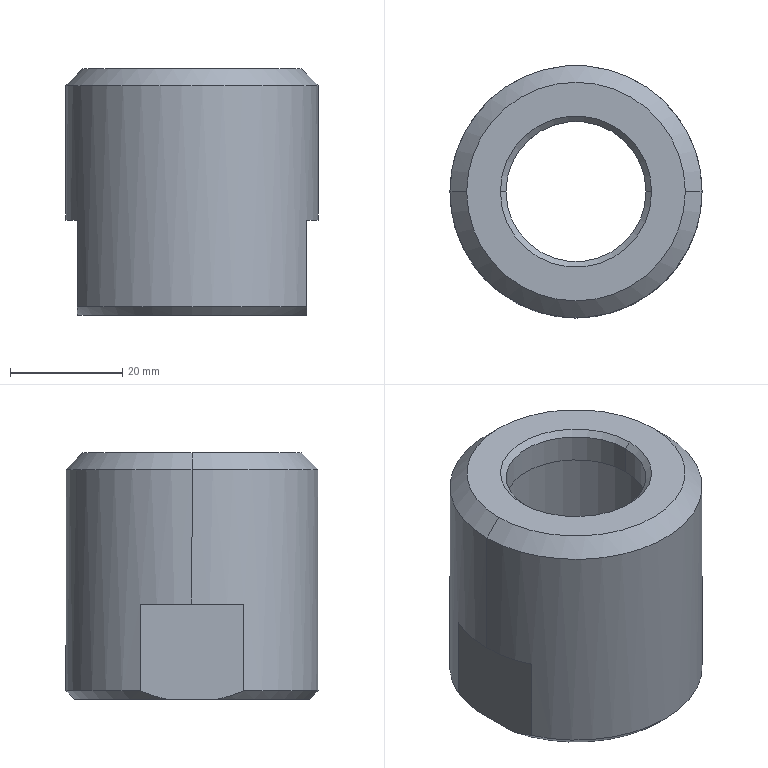Part | SolidWorks | features BaseBody 1 | 1 solid | 24 faces | box 45 x 45 x 44 mm | volume 29973 mm3 | cylinder 8 | cone 8 | plane 8 | commonest cylinder face diameters 25 x2 34.376 x2 34.5 x2 45 x2
STEP:
#1=CARTESIAN_POINT('',(-20.5,9.274,-27.));
#2=VERTEX_POINT('',#1);
#3=CARTESIAN_POINT('',(-22.5,0.,-27.));
#4=VERTEX_POINT('',#3);
#5=CARTESIAN_POINT('',(0.,0.,-27.));
#6=DIRECTION('',(0.,0.,1.));
#7=DIRECTION('',(1.,0.,0.));
#8=AXIS2_PLACEMENT_3D('',#5,#6,#7);
#9=CIRCLE('',#8,22.5);
#10=EDGE_CURVE('',#2,#4,#9,.T.);
#11=ORIENTED_EDGE('',*,*,#10,.T.);
#12=CARTESIAN_POINT('',(-22.5,0.,-3.));
#13=VERTEX_POINT('',#12);
#14=CARTESIAN_POINT('',(-22.5,0.,-44.));
#15=DIRECTION('',(0.,0.,1.));
#16=VECTOR('',#15,1000.);
#17=LINE('',#14,#16);
#18=EDGE_CURVE('',#4,#13,#17,.T.);
#19=ORIENTED_EDGE('',*,*,#18,.T.);
#20=CARTESIAN_POINT('',(22.5,0.,-3.));
#21=VERTEX_POINT('',#20);
#22=CARTESIAN_POINT('',(0.,0.,-3.));
#23=DIRECTION('',(0.,0.,-1.));
#24=DIRECTION('',(1.,0.,0.));
#25=AXIS2_PLACEMENT_3D('',#22,#23,#24);
#26=CIRCLE('',#25,22.5);
#27=EDGE_CURVE('',#13,#21,#26,.T.);
#28=ORIENTED_EDGE('',*,*,#27,.T.);
#29=CARTESIAN_POINT('',(22.5,0.,-27.));
#30=VERTEX_POINT('',#29);
#31=CARTESIAN_POINT('',(22.5,0.,-44.));
#32=DIRECTION('',(0.,0.,1.));
#33=VECTOR('',#32,1000.);
#34=LINE('',#31,#33);
#35=EDGE_CURVE('',#30,#21,#34,.T.);
#36=ORIENTED_EDGE('',*,*,#35,.F.);
#37=CARTESIAN_POINT('',(20.5,9.274,-27.));
#38=VERTEX_POINT('',#37);
#39=CARTESIAN_POINT('',(0.,0.,-27.));
#40=DIRECTION('',(0.,0.,1.));
#41=DIRECTION('',(1.,0.,0.));
#42=AXIS2_PLACEMENT_3D('',#39,#40,#41);
#43=CIRCLE('',#42,22.5);
#44=EDGE_CURVE('',#30,#38,#43,.T.);
#45=ORIENTED_EDGE('',*,*,#44,.T.);
#46=CARTESIAN_POINT('',(20.5,9.274,-42.5));
#47=VERTEX_POINT('',#46);
#48=CARTESIAN_POINT('',(20.5,9.274,-44.));
#49=DIRECTION('',(0.,0.,-1.));
#50=VECTOR('',#49,1000.);
#51=LINE('',#48,#50);
#52=EDGE_CURVE('',#38,#47,#51,.T.);
#53=ORIENTED_EDGE('',*,*,#52,.T.);
#54=CARTESIAN_POINT('',(-20.5,9.274,-42.5));
#55=VERTEX_POINT('',#54);
#56=CARTESIAN_POINT('',(0.,0.,-42.5));
#57=DIRECTION('',(0.,0.,1.));
#58=DIRECTION('',(1.,0.,0.));
#59=AXIS2_PLACEMENT_3D('',#56,#57,#58);
#60=CIRCLE('',#59,22.5);
#61=EDGE_CURVE('',#47,#55,#60,.T.);
#62=ORIENTED_EDGE('',*,*,#61,.T.);
#63=CARTESIAN_POINT('',(-20.5,9.274,-44.));
#64=DIRECTION('',(0.,0.,1.));
#65=VECTOR('',#64,1000.);
#66=LINE('',#63,#65);
#67=EDGE_CURVE('',#55,#2,#66,.T.);
#68=ORIENTED_EDGE('',*,*,#67,.T.);
#69=EDGE_LOOP('',(#11,#19,#28,#36,#45,#53,#62,#68));
#70=FACE_OUTER_BOUND('',#69,.T.);
#71=CARTESIAN_POINT('',(0.,0.,-44.));
#72=DIRECTION('',(0.,0.,1.));
#73=DIRECTION('',(1.,0.,0.));
#74=AXIS2_PLACEMENT_3D('',#71,#72,#73);
#75=CYLINDRICAL_SURFACE('',#74,22.5);
#76=ADVANCED_FACE('',(#70),#75,.T.);
#77=CARTESIAN_POINT('',(-19.5,0.,0.));
#78=VERTEX_POINT('',#77);
#79=CARTESIAN_POINT('',(19.5,0.,0.));
#80=VERTEX_POINT('',#79);
#81=CARTESIAN_POINT('',(0.,0.,0.));
#82=DIRECTION('',(0.,0.,-1.));
#83=DIRECTION('',(-1.,0.,0.));
#84=AXIS2_PLACEMENT_3D('',#81,#82,#83);
#85=CIRCLE('',#84,19.5);
#86=EDGE_CURVE('',#78,#80,#85,.T.);
#87=ORIENTED_EDGE('',*,*,#86,.T.);
#88=CARTESIAN_POINT('',(22.5,0.,-3.));
#89=DIRECTION('',(0.7071,0.,-0.7071));
#90=VECTOR('',#89,1000.);
#91=LINE('',#88,#90);
#92=EDGE_CURVE('',#80,#21,#91,.T.);
#93=ORIENTED_EDGE('',*,*,#92,.T.);
#94=ORIENTED_EDGE('',*,*,#27,.F.);
#95=CARTESIAN_POINT('',(-22.5,0.,-3.));
#96=DIRECTION('',(-0.7071,0.,-0.7071));
#97=VECTOR('',#96,1000.);
#98=LINE('',#95,#97);
#99=EDGE_CURVE('',#78,#13,#98,.T.);
#100=ORIENTED_EDGE('',*,*,#99,.F.);
#101=EDGE_LOOP('',(#87,#93,#94,#100));
#102=FACE_OUTER_BOUND('',#101,.T.);
#103=CARTESIAN_POINT('',(0.,0.,-3.));
#104=DIRECTION('',(0.,0.,-1.));
#105=DIRECTION('',(-1.,0.,0.));
#106=AXIS2_PLACEMENT_3D('',#103,#104,#105);
#107=CONICAL_SURFACE('',#106,22.5,0.7854);
#108=ADVANCED_FACE('',(#102),#107,.T.);
#109=CARTESIAN_POINT('',(17.188,0.,-43.188));
#110=VERTEX_POINT('',#109);
#111=CARTESIAN_POINT('',(-17.188,0.,-43.188));
#112=VERTEX_POINT('',#111);
#113=CARTESIAN_POINT('',(0.,0.,-43.188));
#114=DIRECTION('',(0.,0.,-1.));
#115=DIRECTION('',(-1.,0.,0.));
#116=AXIS2_PLACEMENT_3D('',#113,#114,#115);
#117=CIRCLE('',#116,17.188);
#118=EDGE_CURVE('',#110,#112,#117,.T.);
#119=ORIENTED_EDGE('',*,*,#118,.F.);
#120=CARTESIAN_POINT('',(18.,0.,-44.));
#121=VERTEX_POINT('',#120);
#122=CARTESIAN_POINT('',(18.,0.,-44.));
#123=DIRECTION('',(0.7071,0.,-0.7071));
#124=VECTOR('',#123,1000.);
#125=LINE('',#122,#124);
#126=EDGE_CURVE('',#110,#121,#125,.T.);
#127=ORIENTED_EDGE('',*,*,#126,.T.);
#128=CARTESIAN_POINT('',(-18.,0.,-44.));
#129=VERTEX_POINT('',#128);
#130=CARTESIAN_POINT('',(0.,0.,-44.));
#131=DIRECTION('',(0.,0.,1.));
#132=DIRECTION('',(-1.,0.,0.));
#133=AXIS2_PLACEMENT_3D('',#130,#131,#132);
#134=CIRCLE('',#133,18.);
#135=EDGE_CURVE('',#129,#121,#134,.T.);
#136=ORIENTED_EDGE('',*,*,#135,.F.);
#137=CARTESIAN_POINT('',(-18.,0.,-44.));
#138=DIRECTION('',(-0.7071,0.,-0.7071));
#139=VECTOR('',#138,1000.);
#140=LINE('',#137,#139);
#141=EDGE_CURVE('',#112,#129,#140,.T.);
#142=ORIENTED_EDGE('',*,*,#141,.F.);
#143=EDGE_LOOP('',(#119,#127,#136,#142));
#144=FACE_OUTER_BOUND('',#143,.T.);
#145=CARTESIAN_POINT('',(0.,0.,-44.));
#146=DIRECTION('',(0.,0.,-1.));
#147=DIRECTION('',(-1.,0.,0.));
#148=AXIS2_PLACEMENT_3D('',#145,#146,#147);
#149=CONICAL_SURFACE('',#148,18.,0.7854);
#150=ADVANCED_FACE('',(#144),#149,.F.);
#151=CARTESIAN_POINT('',(-12.5,0.,-1.));
#152=VERTEX_POINT('',#151);
#153=CARTESIAN_POINT('',(12.5,0.,-1.));
#154=VERTEX_POINT('',#153);
#155=CARTESIAN_POINT('',(0.,0.,-1.));
#156=DIRECTION('',(0.,0.,1.));
#157=DIRECTION('',(1.,0.,0.));
#158=AXIS2_PLACEMENT_3D('',#155,#156,#157);
#159=CIRCLE('',#158,12.5);
#160=EDGE_CURVE('',#152,#154,#159,.T.);
#161=ORIENTED_EDGE('',*,*,#160,.F.);
#162=CARTESIAN_POINT('',(-13.5,0.,0.));
#163=VERTEX_POINT('',#162);
#164=CARTESIAN_POINT('',(-13.5,0.,0.));
#165=DIRECTION('',(-0.7071,0.,0.7071));
#166=VECTOR('',#165,1000.);
#167=LINE('',#164,#166);
#168=EDGE_CURVE('',#152,#163,#167,.T.);
#169=ORIENTED_EDGE('',*,*,#168,.T.);
#170=CARTESIAN_POINT('',(13.5,0.,0.));
#171=VERTEX_POINT('',#170);
#172=CARTESIAN_POINT('',(0.,0.,0.));
#173=DIRECTION('',(0.,0.,-1.));
#174=DIRECTION('',(1.,0.,0.));
#175=AXIS2_PLACEMENT_3D('',#172,#173,#174);
#176=CIRCLE('',#175,13.5);
#177=EDGE_CURVE('',#171,#163,#176,.T.);
#178=ORIENTED_EDGE('',*,*,#177,.F.);
#179=CARTESIAN_POINT('',(13.5,0.,0.));
#180=DIRECTION('',(0.7071,0.,0.7071));
#181=VECTOR('',#180,1000.);
#182=LINE('',#179,#181);
#183=EDGE_CURVE('',#154,#171,#182,.T.);
#184=ORIENTED_EDGE('',*,*,#183,.F.);
#185=EDGE_LOOP('',(#161,#169,#178,#184));
#186=FACE_OUTER_BOUND('',#185,.T.);
#187=CARTESIAN_POINT('',(0.,0.,0.));
#188=DIRECTION('',(0.,0.,1.));
#189=DIRECTION('',(1.,0.,0.));
#190=AXIS2_PLACEMENT_3D('',#187,#188,#189);
#191=CONICAL_SURFACE('',#190,13.5,0.7854);
#192=ADVANCED_FACE('',(#186),#191,.F.);
#193=ORIENTED_EDGE('',*,*,#118,.T.);
#194=CARTESIAN_POINT('',(-17.188,0.,-27.));
#195=VERTEX_POINT('',#194);
#196=CARTESIAN_POINT('',(-17.188,0.,-44.));
#197=DIRECTION('',(0.,0.,1.));
#198=VECTOR('',#197,1000.);
#199=LINE('',#196,#198);
#200=EDGE_CURVE('',#112,#195,#199,.T.);
#201=ORIENTED_EDGE('',*,*,#200,.T.);
#202=CARTESIAN_POINT('',(17.188,0.,-27.));
#203=VERTEX_POINT('',#202);
#204=CARTESIAN_POINT('',(0.,0.,-27.));
#205=DIRECTION('',(0.,0.,-1.));
#206=DIRECTION('',(1.,0.,0.));
#207=AXIS2_PLACEMENT_3D('',#204,#205,#206);
#208=CIRCLE('',#207,17.188);
#209=EDGE_CURVE('',#203,#195,#208,.T.);
#210=ORIENTED_EDGE('',*,*,#209,.F.);
#211=CARTESIAN_POINT('',(17.188,0.,-44.));
#212=DIRECTION('',(0.,0.,1.));
#213=VECTOR('',#212,1000.);
#214=LINE('',#211,#213);
#215=EDGE_CURVE('',#110,#203,#214,.T.);
#216=ORIENTED_EDGE('',*,*,#215,.F.);
#217=EDGE_LOOP('',(#193,#201,#210,#216));
#218=FACE_OUTER_BOUND('',#217,.T.);
#219=CARTESIAN_POINT('',(0.,0.,-44.));
#220=DIRECTION('',(0.,0.,1.));
#221=DIRECTION('',(1.,0.,0.));
#222=AXIS2_PLACEMENT_3D('',#219,#220,#221);
#223=CYLINDRICAL_SURFACE('',#222,17.188);
#224=ADVANCED_FACE('',(#218),#223,.F.);
#225=CARTESIAN_POINT('',(-12.5,0.,-6.));
#226=VERTEX_POINT('',#225);
#227=CARTESIAN_POINT('',(12.5,0.,-6.));
#228=VERTEX_POINT('',#227);
#229=CARTESIAN_POINT('',(0.,0.,-6.));
#230=DIRECTION('',(0.,0.,1.));
#231=DIRECTION('',(1.,0.,0.));
#232=AXIS2_PLACEMENT_3D('',#229,#230,#231);
#233=CIRCLE('',#232,12.5);
#234=EDGE_CURVE('',#226,#228,#233,.T.);
#235=ORIENTED_EDGE('',*,*,#234,.F.);
#236=CARTESIAN_POINT('',(-12.5,0.,-44.));
#237=DIRECTION('',(0.,0.,1.));
#238=VECTOR('',#237,1000.);
#239=LINE('',#236,#238);
#240=EDGE_CURVE('',#226,#152,#239,.T.);
#241=ORIENTED_EDGE('',*,*,#240,.T.);
#242=ORIENTED_EDGE('',*,*,#160,.T.);
#243=CARTESIAN_POINT('',(12.5,0.,-44.));
#244=DIRECTION('',(0.,0.,1.));
#245=VECTOR('',#244,1000.);
#246=LINE('',#243,#245);
#247=EDGE_CURVE('',#228,#154,#246,.T.);
#248=ORIENTED_EDGE('',*,*,#247,.F.);
#249=EDGE_LOOP('',(#235,#241,#242,#248));
#250=FACE_OUTER_BOUND('',#249,.T.);
#251=CARTESIAN_POINT('',(0.,0.,-44.));
#252=DIRECTION('',(0.,0.,1.));
#253=DIRECTION('',(1.,0.,0.));
#254=AXIS2_PLACEMENT_3D('',#251,#252,#253);
#255=CYLINDRICAL_SURFACE('',#254,12.5);
#256=ADVANCED_FACE('',(#250),#255,.F.);
#257=CARTESIAN_POINT('',(-17.25,0.,-27.));
#258=VERTEX_POINT('',#257);
#259=CARTESIAN_POINT('',(17.25,0.,-27.));
#260=VERTEX_POINT('',#259);
#261=CARTESIAN_POINT('',(0.,0.,-27.));
#262=DIRECTION('',(0.,0.,1.));
#263=DIRECTION('',(1.,0.,0.));
#264=AXIS2_PLACEMENT_3D('',#261,#262,#263);
#265=CIRCLE('',#264,17.25);
#266=EDGE_CURVE('',#258,#260,#265,.T.);
#267=ORIENTED_EDGE('',*,*,#266,.F.);
#268=CARTESIAN_POINT('',(-17.25,0.,-6.));
#269=VERTEX_POINT('',#268);
#270=CARTESIAN_POINT('',(-17.25,0.,-44.));
#271=DIRECTION('',(0.,0.,1.));
#272=VECTOR('',#271,1000.);
#273=LINE('',#270,#272);
#274=EDGE_CURVE('',#258,#269,#273,.T.);
#275=ORIENTED_EDGE('',*,*,#274,.T.);
#276=CARTESIAN_POINT('',(17.25,0.,-6.));
#277=VERTEX_POINT('',#276);
#278=CARTESIAN_POINT('',(0.,0.,-6.));
#279=DIRECTION('',(0.,0.,-1.));
#280=DIRECTION('',(1.,0.,0.));
#281=AXIS2_PLACEMENT_3D('',#278,#279,#280);
#282=CIRCLE('',#281,17.25);
#283=EDGE_CURVE('',#277,#269,#282,.T.);
#284=ORIENTED_EDGE('',*,*,#283,.F.);
#285=CARTESIAN_POINT('',(17.25,0.,-44.));
#286=DIRECTION('',(0.,0.,1.));
#287=VECTOR('',#286,1000.);
#288=LINE('',#285,#287);
#289=EDGE_CURVE('',#260,#277,#288,.T.);
#290=ORIENTED_EDGE('',*,*,#289,.F.);
#291=EDGE_LOOP('',(#267,#275,#284,#290));
#292=FACE_OUTER_BOUND('',#291,.T.);
#293=CARTESIAN_POINT('',(0.,0.,-44.));
#294=DIRECTION('',(0.,0.,1.));
#295=DIRECTION('',(1.,0.,0.));
#296=AXIS2_PLACEMENT_3D('',#293,#294,#295);
#297=CYLINDRICAL_SURFACE('',#296,17.25);
#298=ADVANCED_FACE('',(#292),#297,.F.);
#299=ORIENTED_EDGE('',*,*,#18,.F.);
#300=CARTESIAN_POINT('',(-20.5,-9.274,-27.));
#301=VERTEX_POINT('',#300);
#302=CARTESIAN_POINT('',(0.,0.,-27.));
#303=DIRECTION('',(0.,0.,1.));
#304=DIRECTION('',(1.,0.,0.));
#305=AXIS2_PLACEMENT_3D('',#302,#303,#304);
#306=CIRCLE('',#305,22.5);
#307=EDGE_CURVE('',#4,#301,#306,.T.);
#308=ORIENTED_EDGE('',*,*,#307,.T.);
#309=CARTESIAN_POINT('',(-20.5,-9.274,-42.5));
#310=VERTEX_POINT('',#309);
#311=CARTESIAN_POINT('',(-20.5,-9.274,-44.));
#312=DIRECTION('',(0.,0.,-1.));
#313=VECTOR('',#312,1000.);
#314=LINE('',#311,#313);
#315=EDGE_CURVE('',#301,#310,#314,.T.);
#316=ORIENTED_EDGE('',*,*,#315,.T.);
#317=CARTESIAN_POINT('',(20.5,-9.274,-42.5));
#318=VERTEX_POINT('',#317);
#319=CARTESIAN_POINT('',(0.,0.,-42.5));
#320=DIRECTION('',(0.,0.,1.));
#321=DIRECTION('',(1.,0.,0.));
#322=AXIS2_PLACEMENT_3D('',#319,#320,#321);
#323=CIRCLE('',#322,22.5);
#324=EDGE_CURVE('',#310,#318,#323,.T.);
#325=ORIENTED_EDGE('',*,*,#324,.T.);
#326=CARTESIAN_POINT('',(20.5,-9.274,-27.));
#327=VERTEX_POINT('',#326);
#328=CARTESIAN_POINT('',(20.5,-9.274,-44.));
#329=DIRECTION('',(0.,0.,1.));
#330=VECTOR('',#329,1000.);
#331=LINE('',#328,#330);
#332=EDGE_CURVE('',#318,#327,#331,.T.);
#333=ORIENTED_EDGE('',*,*,#332,.T.);
#334=CARTESIAN_POINT('',(0.,0.,-27.));
#335=DIRECTION('',(0.,0.,1.));
#336=DIRECTION('',(1.,0.,0.));
#337=AXIS2_PLACEMENT_3D('',#334,#335,#336);
#338=CIRCLE('',#337,22.5);
#339=EDGE_CURVE('',#327,#30,#338,.T.);
#340=ORIENTED_EDGE('',*,*,#339,.T.);
#341=ORIENTED_EDGE('',*,*,#35,.T.);
#342=CARTESIAN_POINT('',(0.,0.,-3.));
#343=DIRECTION('',(0.,0.,-1.));
#344=DIRECTION('',(1.,0.,0.));
#345=AXIS2_PLACEMENT_3D('',#342,#343,#344);
#346=CIRCLE('',#345,22.5);
#347=EDGE_CURVE('',#21,#13,#346,.T.);
#348=ORIENTED_EDGE('',*,*,#347,.T.);
#349=EDGE_LOOP('',(#299,#308,#316,#325,#333,#340,#341,#348));
#350=FACE_OUTER_BOUND('',#349,.T.);
#351=CARTESIAN_POINT('',(0.,0.,-44.));
#352=DIRECTION('',(0.,0.,1.));
#353=DIRECTION('',(1.,0.,0.));
#354=AXIS2_PLACEMENT_3D('',#351,#352,#353);
#355=CYLINDRICAL_SURFACE('',#354,22.5);
#356=ADVANCED_FACE('',(#350),#355,.T.);
#357=CARTESIAN_POINT('',(20.5,30.,-27.));
#358=DIRECTION('',(0.,-1.,0.));
#359=VECTOR('',#358,1000.);
#360=LINE('',#357,#359);
#361=EDGE_CURVE('',#38,#327,#360,.T.);
#362=ORIENTED_EDGE('',*,*,#361,.T.);
#363=ORIENTED_EDGE('',*,*,#332,.F.);
#364=CARTESIAN_POINT('',(20.5,-4.555,-44.));
#365=VERTEX_POINT('',#364);
#366=CARTESIAN_POINT('',(20.5,-9.274,-42.5));
#367=CARTESIAN_POINT('',(20.5,-7.742,-43.131));
#368=CARTESIAN_POINT('',(20.5,-6.175,-43.649));
#369=CARTESIAN_POINT('',(20.5,-4.555,-44.));
#370=B_SPLINE_CURVE_WITH_KNOTS('',3,(#366,#367,#368,#369),.UNSPECIFIED.,.F.,.F.,(4,4),(0.,0.004951),.UNSPECIFIED.);
#371=EDGE_CURVE('',#318,#365,#370,.T.);
#372=ORIENTED_EDGE('',*,*,#371,.T.);
#373=CARTESIAN_POINT('',(20.5,4.555,-44.));
#374=VERTEX_POINT('',#373);
#375=CARTESIAN_POINT('',(20.5,30.,-44.));
#376=DIRECTION('',(0.,1.,0.));
#377=VECTOR('',#376,1000.);
#378=LINE('',#375,#377);
#379=EDGE_CURVE('',#365,#374,#378,.T.);
#380=ORIENTED_EDGE('',*,*,#379,.T.);
#381=CARTESIAN_POINT('',(20.5,4.555,-44.));
#382=CARTESIAN_POINT('',(20.5,6.175,-43.649));
#383=CARTESIAN_POINT('',(20.5,7.742,-43.131));
#384=CARTESIAN_POINT('',(20.5,9.274,-42.5));
#385=B_SPLINE_CURVE_WITH_KNOTS('',3,(#381,#382,#383,#384),.UNSPECIFIED.,.F.,.F.,(4,4),(0.,0.004951),.UNSPECIFIED.);
#386=EDGE_CURVE('',#374,#47,#385,.T.);
#387=ORIENTED_EDGE('',*,*,#386,.T.);
#388=ORIENTED_EDGE('',*,*,#52,.F.);
#389=EDGE_LOOP('',(#362,#363,#372,#380,#387,#388));
#390=FACE_OUTER_BOUND('',#389,.T.);
#391=CARTESIAN_POINT('',(20.5,30.,-47.));
#392=DIRECTION('',(1.,0.,0.));
#393=DIRECTION('',(0.,0.,-1.));
#394=AXIS2_PLACEMENT_3D('',#391,#392,#393);
#395=PLANE('',#394);
#396=ADVANCED_FACE('',(#390),#395,.T.);
#397=ORIENTED_EDGE('',*,*,#361,.F.);
#398=ORIENTED_EDGE('',*,*,#44,.F.);
#399=ORIENTED_EDGE('',*,*,#339,.F.);
#400=EDGE_LOOP('',(#397,#398,#399));
#401=FACE_OUTER_BOUND('',#400,.T.);
#402=CARTESIAN_POINT('',(20.5,30.,-27.));
#403=DIRECTION('',(0.,0.,-1.));
#404=DIRECTION('',(-1.,0.,0.));
#405=AXIS2_PLACEMENT_3D('',#402,#403,#404);
#406=PLANE('',#405);
#407=ADVANCED_FACE('',(#401),#406,.T.);
#408=CARTESIAN_POINT('',(-20.5,-4.555,-44.));
#409=VERTEX_POINT('',#408);
#410=CARTESIAN_POINT('',(0.,0.,-44.));
#411=DIRECTION('',(0.,0.,1.));
#412=DIRECTION('',(1.,0.,0.));
#413=AXIS2_PLACEMENT_3D('',#410,#411,#412);
#414=CIRCLE('',#413,21.);
#415=EDGE_CURVE('',#409,#365,#414,.T.);
#416=ORIENTED_EDGE('',*,*,#415,.T.);
#417=ORIENTED_EDGE('',*,*,#371,.F.);
#418=ORIENTED_EDGE('',*,*,#324,.F.);
#419=CARTESIAN_POINT('',(-20.5,-9.274,-42.5));
#420=CARTESIAN_POINT('',(-20.5,-7.742,-43.131));
#421=CARTESIAN_POINT('',(-20.5,-6.175,-43.649));
#422=CARTESIAN_POINT('',(-20.5,-4.555,-44.));
#423=B_SPLINE_CURVE_WITH_KNOTS('',3,(#419,#420,#421,#422),.UNSPECIFIED.,.F.,.F.,(4,4),(0.,0.004951),.UNSPECIFIED.);
#424=EDGE_CURVE('',#310,#409,#423,.T.);
#425=ORIENTED_EDGE('',*,*,#424,.T.);
#426=EDGE_LOOP('',(#416,#417,#418,#425));
#427=FACE_OUTER_BOUND('',#426,.T.);
#428=CARTESIAN_POINT('',(0.,0.,-42.5));
#429=DIRECTION('',(0.,0.,1.));
#430=DIRECTION('',(1.,0.,0.));
#431=AXIS2_PLACEMENT_3D('',#428,#429,#430);
#432=CONICAL_SURFACE('',#431,22.5,0.7854);
#433=ADVANCED_FACE('',(#427),#432,.T.);
#434=CARTESIAN_POINT('',(-20.5,30.,-27.));
#435=DIRECTION('',(0.,1.,0.));
#436=VECTOR('',#435,1000.);
#437=LINE('',#434,#436);
#438=EDGE_CURVE('',#301,#2,#437,.T.);
#439=ORIENTED_EDGE('',*,*,#438,.T.);
#440=ORIENTED_EDGE('',*,*,#67,.F.);
#441=CARTESIAN_POINT('',(-20.5,4.555,-44.));
#442=VERTEX_POINT('',#441);
#443=CARTESIAN_POINT('',(-20.5,9.274,-42.5));
#444=CARTESIAN_POINT('',(-20.5,7.742,-43.131));
#445=CARTESIAN_POINT('',(-20.5,6.175,-43.649));
#446=CARTESIAN_POINT('',(-20.5,4.555,-44.));
#447=B_SPLINE_CURVE_WITH_KNOTS('',3,(#443,#444,#445,#446),.UNSPECIFIED.,.F.,.F.,(4,4),(0.,0.004951),.UNSPECIFIED.);
#448=EDGE_CURVE('',#55,#442,#447,.T.);
#449=ORIENTED_EDGE('',*,*,#448,.T.);
#450=CARTESIAN_POINT('',(-20.5,30.,-44.));
#451=DIRECTION('',(0.,-1.,0.));
#452=VECTOR('',#451,1000.);
#453=LINE('',#450,#452);
#454=EDGE_CURVE('',#442,#409,#453,.T.);
#455=ORIENTED_EDGE('',*,*,#454,.T.);
#456=ORIENTED_EDGE('',*,*,#424,.F.);
#457=ORIENTED_EDGE('',*,*,#315,.F.);
#458=EDGE_LOOP('',(#439,#440,#449,#455,#456,#457));
#459=FACE_OUTER_BOUND('',#458,.T.);
#460=CARTESIAN_POINT('',(-20.5,30.,-27.));
#461=DIRECTION('',(-1.,0.,0.));
#462=DIRECTION('',(0.,0.,1.));
#463=AXIS2_PLACEMENT_3D('',#460,#461,#462);
#464=PLANE('',#463);
#465=ADVANCED_FACE('',(#459),#464,.T.);
#466=ORIENTED_EDGE('',*,*,#438,.F.);
#467=ORIENTED_EDGE('',*,*,#307,.F.);
#468=ORIENTED_EDGE('',*,*,#10,.F.);
#469=EDGE_LOOP('',(#466,#467,#468));
#470=FACE_OUTER_BOUND('',#469,.T.);
#471=CARTESIAN_POINT('',(-50.,30.,-27.));
#472=DIRECTION('',(0.,0.,-1.));
#473=DIRECTION('',(-1.,0.,0.));
#474=AXIS2_PLACEMENT_3D('',#471,#472,#473);
#475=PLANE('',#474);
#476=ADVANCED_FACE('',(#470),#475,.T.);
#477=CARTESIAN_POINT('',(0.,0.,-44.));
#478=DIRECTION('',(0.,0.,1.));
#479=DIRECTION('',(1.,0.,0.));
#480=AXIS2_PLACEMENT_3D('',#477,#478,#479);
#481=CIRCLE('',#480,21.);
#482=EDGE_CURVE('',#374,#442,#481,.T.);
#483=ORIENTED_EDGE('',*,*,#482,.T.);
#484=ORIENTED_EDGE('',*,*,#448,.F.);
#485=ORIENTED_EDGE('',*,*,#61,.F.);
#486=ORIENTED_EDGE('',*,*,#386,.F.);
#487=EDGE_LOOP('',(#483,#484,#485,#486));
#488=FACE_OUTER_BOUND('',#487,.T.);
#489=CARTESIAN_POINT('',(0.,0.,-42.5));
#490=DIRECTION('',(0.,0.,1.));
#491=DIRECTION('',(1.,0.,0.));
#492=AXIS2_PLACEMENT_3D('',#489,#490,#491);
#493=CONICAL_SURFACE('',#492,22.5,0.7854);
#494=ADVANCED_FACE('',(#488),#493,.T.);
#495=ORIENTED_EDGE('',*,*,#92,.F.);
#496=CARTESIAN_POINT('',(0.,0.,0.));
#497=DIRECTION('',(0.,0.,-1.));
#498=DIRECTION('',(-1.,0.,0.));
#499=AXIS2_PLACEMENT_3D('',#496,#497,#498);
#500=CIRCLE('',#499,19.5);
#501=EDGE_CURVE('',#80,#78,#500,.T.);
#502=ORIENTED_EDGE('',*,*,#501,.T.);
#503=ORIENTED_EDGE('',*,*,#99,.T.);
#504=ORIENTED_EDGE('',*,*,#347,.F.);
#505=EDGE_LOOP('',(#495,#502,#503,#504));
#506=FACE_OUTER_BOUND('',#505,.T.);
#507=CARTESIAN_POINT('',(0.,0.,-3.));
#508=DIRECTION('',(0.,0.,-1.));
#509=DIRECTION('',(-1.,0.,0.));
#510=AXIS2_PLACEMENT_3D('',#507,#508,#509);
#511=CONICAL_SURFACE('',#510,22.5,0.7854);
#512=ADVANCED_FACE('',(#506),#511,.T.);
#513=ORIENTED_EDGE('',*,*,#135,.T.);
#514=CARTESIAN_POINT('',(0.,0.,-44.));
#515=DIRECTION('',(0.,0.,1.));
#516=DIRECTION('',(-1.,0.,0.));
#517=AXIS2_PLACEMENT_3D('',#514,#515,#516);
#518=CIRCLE('',#517,18.);
#519=EDGE_CURVE('',#121,#129,#518,.T.);
#520=ORIENTED_EDGE('',*,*,#519,.T.);
#521=EDGE_LOOP('',(#513,#520));
#522=FACE_BOUND('',#521,.T.);
#523=ORIENTED_EDGE('',*,*,#379,.F.);
#524=ORIENTED_EDGE('',*,*,#415,.F.);
#525=ORIENTED_EDGE('',*,*,#454,.F.);
#526=ORIENTED_EDGE('',*,*,#482,.F.);
#527=EDGE_LOOP('',(#523,#524,#525,#526));
#528=FACE_OUTER_BOUND('',#527,.T.);
#529=CARTESIAN_POINT('',(0.,18.,-44.));
#530=DIRECTION('',(0.,0.,-1.));
#531=DIRECTION('',(-1.,0.,0.));
#532=AXIS2_PLACEMENT_3D('',#529,#530,#531);
#533=PLANE('',#532);
#534=ADVANCED_FACE('',(#522,#528),#533,.T.);
#535=ORIENTED_EDGE('',*,*,#86,.F.);
#536=ORIENTED_EDGE('',*,*,#501,.F.);
#537=EDGE_LOOP('',(#535,#536));
#538=FACE_OUTER_BOUND('',#537,.T.);
#539=ORIENTED_EDGE('',*,*,#177,.T.);
#540=CARTESIAN_POINT('',(0.,0.,0.));
#541=DIRECTION('',(0.,0.,-1.));
#542=DIRECTION('',(1.,0.,0.));
#543=AXIS2_PLACEMENT_3D('',#540,#541,#542);
#544=CIRCLE('',#543,13.5);
#545=EDGE_CURVE('',#163,#171,#544,.T.);
#546=ORIENTED_EDGE('',*,*,#545,.T.);
#547=EDGE_LOOP('',(#539,#546));
#548=FACE_BOUND('',#547,.T.);
#549=CARTESIAN_POINT('',(0.,19.5,0.));
#550=DIRECTION('',(0.,0.,1.));
#551=DIRECTION('',(1.,0.,0.));
#552=AXIS2_PLACEMENT_3D('',#549,#550,#551);
#553=PLANE('',#552);
#554=ADVANCED_FACE('',(#538,#548),#553,.T.);
#555=ORIENTED_EDGE('',*,*,#126,.F.);
#556=CARTESIAN_POINT('',(0.,0.,-43.188));
#557=DIRECTION('',(0.,0.,-1.));
#558=DIRECTION('',(-1.,0.,0.));
#559=AXIS2_PLACEMENT_3D('',#556,#557,#558);
#560=CIRCLE('',#559,17.188);
#561=EDGE_CURVE('',#112,#110,#560,.T.);
#562=ORIENTED_EDGE('',*,*,#561,.F.);
#563=ORIENTED_EDGE('',*,*,#141,.T.);
#564=ORIENTED_EDGE('',*,*,#519,.F.);
#565=EDGE_LOOP('',(#555,#562,#563,#564));
#566=FACE_OUTER_BOUND('',#565,.T.);
#567=CARTESIAN_POINT('',(0.,0.,-44.));
#568=DIRECTION('',(0.,0.,-1.));
#569=DIRECTION('',(-1.,0.,0.));
#570=AXIS2_PLACEMENT_3D('',#567,#568,#569);
#571=CONICAL_SURFACE('',#570,18.,0.7854);
#572=ADVANCED_FACE('',(#566),#571,.F.);
#573=ORIENTED_EDGE('',*,*,#168,.F.);
#574=CARTESIAN_POINT('',(0.,0.,-1.));
#575=DIRECTION('',(0.,0.,1.));
#576=DIRECTION('',(1.,0.,0.));
#577=AXIS2_PLACEMENT_3D('',#574,#575,#576);
#578=CIRCLE('',#577,12.5);
#579=EDGE_CURVE('',#154,#152,#578,.T.);
#580=ORIENTED_EDGE('',*,*,#579,.F.);
#581=ORIENTED_EDGE('',*,*,#183,.T.);
#582=ORIENTED_EDGE('',*,*,#545,.F.);
#583=EDGE_LOOP('',(#573,#580,#581,#582));
#584=FACE_OUTER_BOUND('',#583,.T.);
#585=CARTESIAN_POINT('',(0.,0.,0.));
#586=DIRECTION('',(0.,0.,1.));
#587=DIRECTION('',(1.,0.,0.));
#588=AXIS2_PLACEMENT_3D('',#585,#586,#587);
#589=CONICAL_SURFACE('',#588,13.5,0.7854);
#590=ADVANCED_FACE('',(#584),#589,.F.);
#591=ORIENTED_EDGE('',*,*,#200,.F.);
#592=ORIENTED_EDGE('',*,*,#561,.T.);
#593=ORIENTED_EDGE('',*,*,#215,.T.);
#594=CARTESIAN_POINT('',(0.,0.,-27.));
#595=DIRECTION('',(0.,0.,-1.));
#596=DIRECTION('',(1.,0.,0.));
#597=AXIS2_PLACEMENT_3D('',#594,#595,#596);
#598=CIRCLE('',#597,17.188);
#599=EDGE_CURVE('',#195,#203,#598,.T.);
#600=ORIENTED_EDGE('',*,*,#599,.F.);
#601=EDGE_LOOP('',(#591,#592,#593,#600));
#602=FACE_OUTER_BOUND('',#601,.T.);
#603=CARTESIAN_POINT('',(0.,0.,-44.));
#604=DIRECTION('',(0.,0.,1.));
#605=DIRECTION('',(1.,0.,0.));
#606=AXIS2_PLACEMENT_3D('',#603,#604,#605);
#607=CYLINDRICAL_SURFACE('',#606,17.188);
#608=ADVANCED_FACE('',(#602),#607,.F.);
#609=ORIENTED_EDGE('',*,*,#240,.F.);
#610=CARTESIAN_POINT('',(0.,0.,-6.));
#611=DIRECTION('',(0.,0.,1.));
#612=DIRECTION('',(1.,0.,0.));
#613=AXIS2_PLACEMENT_3D('',#610,#611,#612);
#614=CIRCLE('',#613,12.5);
#615=EDGE_CURVE('',#228,#226,#614,.T.);
#616=ORIENTED_EDGE('',*,*,#615,.F.);
#617=ORIENTED_EDGE('',*,*,#247,.T.);
#618=ORIENTED_EDGE('',*,*,#579,.T.);
#619=EDGE_LOOP('',(#609,#616,#617,#618));
#620=FACE_OUTER_BOUND('',#619,.T.);
#621=CARTESIAN_POINT('',(0.,0.,-44.));
#622=DIRECTION('',(0.,0.,1.));
#623=DIRECTION('',(1.,0.,0.));
#624=AXIS2_PLACEMENT_3D('',#621,#622,#623);
#625=CYLINDRICAL_SURFACE('',#624,12.5);
#626=ADVANCED_FACE('',(#620),#625,.F.);
#627=CARTESIAN_POINT('',(0.,0.,-27.));
#628=DIRECTION('',(0.,0.,1.));
#629=DIRECTION('',(1.,0.,0.));
#630=AXIS2_PLACEMENT_3D('',#627,#628,#629);
#631=CIRCLE('',#630,17.25);
#632=EDGE_CURVE('',#260,#258,#631,.T.);
#633=ORIENTED_EDGE('',*,*,#632,.T.);
#634=ORIENTED_EDGE('',*,*,#266,.T.);
#635=EDGE_LOOP('',(#633,#634));
#636=FACE_OUTER_BOUND('',#635,.T.);
#637=ORIENTED_EDGE('',*,*,#209,.T.);
#638=ORIENTED_EDGE('',*,*,#599,.T.);
#639=EDGE_LOOP('',(#637,#638));
#640=FACE_BOUND('',#639,.T.);
#641=CARTESIAN_POINT('',(0.,17.25,-27.));
#642=DIRECTION('',(0.,0.,1.));
#643=DIRECTION('',(1.,0.,0.));
#644=AXIS2_PLACEMENT_3D('',#641,#642,#643);
#645=PLANE('',#644);
#646=ADVANCED_FACE('',(#636,#640),#645,.T.);
#647=ORIENTED_EDGE('',*,*,#615,.T.);
#648=ORIENTED_EDGE('',*,*,#234,.T.);
#649=EDGE_LOOP('',(#647,#648));
#650=FACE_BOUND('',#649,.T.);
#651=ORIENTED_EDGE('',*,*,#283,.T.);
#652=CARTESIAN_POINT('',(0.,0.,-6.));
#653=DIRECTION('',(0.,0.,-1.));
#654=DIRECTION('',(1.,0.,0.));
#655=AXIS2_PLACEMENT_3D('',#652,#653,#654);
#656=CIRCLE('',#655,17.25);
#657=EDGE_CURVE('',#269,#277,#656,.T.);
#658=ORIENTED_EDGE('',*,*,#657,.T.);
#659=EDGE_LOOP('',(#651,#658));
#660=FACE_OUTER_BOUND('',#659,.T.);
#661=CARTESIAN_POINT('',(0.,12.5,-6.));
#662=DIRECTION('',(0.,0.,-1.));
#663=DIRECTION('',(-1.,0.,0.));
#664=AXIS2_PLACEMENT_3D('',#661,#662,#663);
#665=PLANE('',#664);
#666=ADVANCED_FACE('',(#650,#660),#665,.T.);
#667=ORIENTED_EDGE('',*,*,#274,.F.);
#668=ORIENTED_EDGE('',*,*,#632,.F.);
#669=ORIENTED_EDGE('',*,*,#289,.T.);
#670=ORIENTED_EDGE('',*,*,#657,.F.);
#671=EDGE_LOOP('',(#667,#668,#669,#670));
#672=FACE_OUTER_BOUND('',#671,.T.);
#673=CARTESIAN_POINT('',(0.,0.,-44.));
#674=DIRECTION('',(0.,0.,1.));
#675=DIRECTION('',(1.,0.,0.));
#676=AXIS2_PLACEMENT_3D('',#673,#674,#675);
#677=CYLINDRICAL_SURFACE('',#676,17.25);
#678=ADVANCED_FACE('',(#672),#677,.F.);
#679=CLOSED_SHELL('',(#76,#108,#150,#192,#224,#256,#298,#356,#396,#407,#433,#465,#476,#494,#512,#534,#554,#572,#590,#608,#626,#646,#666,#678));
#680=MANIFOLD_SOLID_BREP('',#679);
#681=CARTESIAN_POINT('',(0.,0.,0.));
#682=DIRECTION('',(0.,0.,1.));
#683=DIRECTION('',(1.,0.,0.));
#684=AXIS2_PLACEMENT_3D('',#681,#682,#683);
#685=(LENGTH_UNIT()NAMED_UNIT(*)SI_UNIT(.MILLI.,.METRE.));
#686=UNCERTAINTY_MEASURE_WITH_UNIT(LENGTH_MEASURE(0.00001),#685,'','');
#687=(NAMED_UNIT(*)PLANE_ANGLE_UNIT()SI_UNIT($,.RADIAN.));
#688=(NAMED_UNIT(*)SI_UNIT($,.STERADIAN.)SOLID_ANGLE_UNIT());
#689=(GEOMETRIC_REPRESENTATION_CONTEXT(3)GLOBAL_UNCERTAINTY_ASSIGNED_CONTEXT((#686))GLOBAL_UNIT_ASSIGNED_CONTEXT((#685,#687,#688))REPRESENTATION_CONTEXT('',''));
#690=ADVANCED_BREP_SHAPE_REPRESENTATION('',(#680,#684),#689);